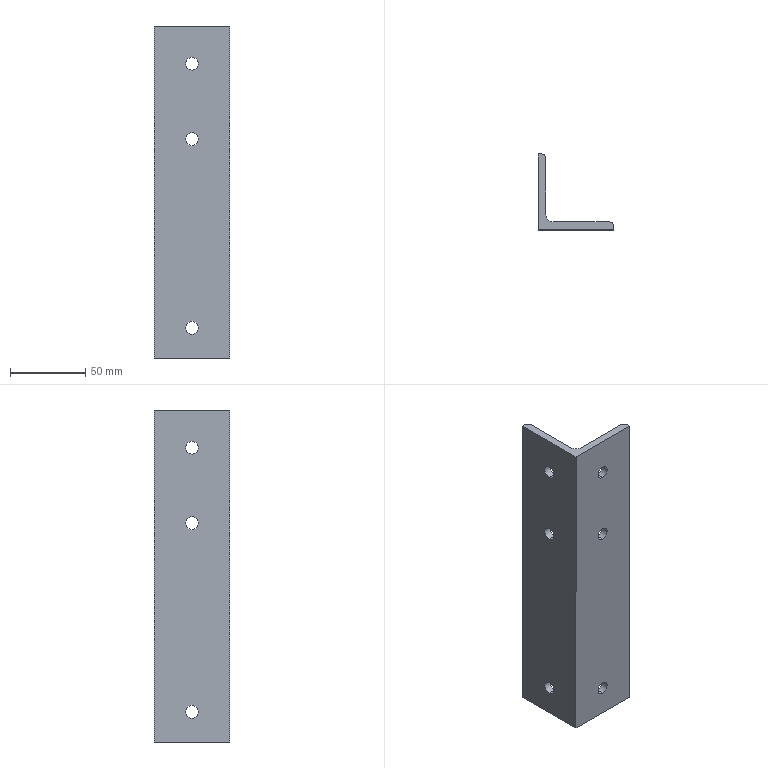Part | STEP file | 750038242 | 1 solid | 23 faces | box 50 x 50 x 220 mm | volume 103128 mm3 | cylinder 15 | plane 8 | commonest cylinder face diameters 8.5 x12 6 x2 10 x1
STEP:
#1=CARTESIAN_POINT('',(5.,25.,-94.25));
#2=VERTEX_POINT('',#1);
#3=CARTESIAN_POINT('',(5.,25.,-85.75));
#4=VERTEX_POINT('',#3);
#5=CARTESIAN_POINT('',(5.,25.,-90.));
#6=DIRECTION('',(-1.,0.,0.));
#7=DIRECTION('',(0.,0.,1.));
#8=AXIS2_PLACEMENT_3D('',#5,#6,#7);
#9=CIRCLE('',#8,4.25);
#10=EDGE_CURVE('',#2,#4,#9,.T.);
#11=ORIENTED_EDGE('',*,*,#10,.F.);
#12=CARTESIAN_POINT('',(0.,25.,-94.25));
#13=VERTEX_POINT('',#12);
#14=CARTESIAN_POINT('',(55.,25.,-94.25));
#15=DIRECTION('',(-1.,0.,0.));
#16=VECTOR('',#15,1000.);
#17=LINE('',#14,#16);
#18=EDGE_CURVE('',#2,#13,#17,.T.);
#19=ORIENTED_EDGE('',*,*,#18,.T.);
#20=CARTESIAN_POINT('',(0.,25.,-85.75));
#21=VERTEX_POINT('',#20);
#22=CARTESIAN_POINT('',(0.,25.,-90.));
#23=DIRECTION('',(-1.,0.,0.));
#24=DIRECTION('',(0.,0.,1.));
#25=AXIS2_PLACEMENT_3D('',#22,#23,#24);
#26=CIRCLE('',#25,4.25);
#27=EDGE_CURVE('',#13,#21,#26,.T.);
#28=ORIENTED_EDGE('',*,*,#27,.T.);
#29=CARTESIAN_POINT('',(55.,25.,-85.75));
#30=DIRECTION('',(-1.,0.,0.));
#31=VECTOR('',#30,1000.);
#32=LINE('',#29,#31);
#33=EDGE_CURVE('',#4,#21,#32,.T.);
#34=ORIENTED_EDGE('',*,*,#33,.F.);
#35=EDGE_LOOP('',(#11,#19,#28,#34));
#36=FACE_OUTER_BOUND('',#35,.T.);
#37=CARTESIAN_POINT('',(55.,25.,-90.));
#38=DIRECTION('',(-1.,0.,0.));
#39=DIRECTION('',(0.,0.,1.));
#40=AXIS2_PLACEMENT_3D('',#37,#38,#39);
#41=CYLINDRICAL_SURFACE('',#40,4.25);
#42=ADVANCED_FACE('',(#36),#41,.F.);
#43=CARTESIAN_POINT('',(5.,25.,30.75));
#44=VERTEX_POINT('',#43);
#45=CARTESIAN_POINT('',(5.,25.,39.25));
#46=VERTEX_POINT('',#45);
#47=CARTESIAN_POINT('',(5.,25.,35.));
#48=DIRECTION('',(-1.,0.,0.));
#49=DIRECTION('',(0.,0.,1.));
#50=AXIS2_PLACEMENT_3D('',#47,#48,#49);
#51=CIRCLE('',#50,4.25);
#52=EDGE_CURVE('',#44,#46,#51,.T.);
#53=ORIENTED_EDGE('',*,*,#52,.F.);
#54=CARTESIAN_POINT('',(0.,25.,30.75));
#55=VERTEX_POINT('',#54);
#56=CARTESIAN_POINT('',(55.,25.,30.75));
#57=DIRECTION('',(-1.,0.,0.));
#58=VECTOR('',#57,1000.);
#59=LINE('',#56,#58);
#60=EDGE_CURVE('',#44,#55,#59,.T.);
#61=ORIENTED_EDGE('',*,*,#60,.T.);
#62=CARTESIAN_POINT('',(0.,25.,39.25));
#63=VERTEX_POINT('',#62);
#64=CARTESIAN_POINT('',(0.,25.,35.));
#65=DIRECTION('',(-1.,0.,0.));
#66=DIRECTION('',(0.,0.,1.));
#67=AXIS2_PLACEMENT_3D('',#64,#65,#66);
#68=CIRCLE('',#67,4.25);
#69=EDGE_CURVE('',#55,#63,#68,.T.);
#70=ORIENTED_EDGE('',*,*,#69,.T.);
#71=CARTESIAN_POINT('',(55.,25.,39.25));
#72=DIRECTION('',(-1.,0.,0.));
#73=VECTOR('',#72,1000.);
#74=LINE('',#71,#73);
#75=EDGE_CURVE('',#46,#63,#74,.T.);
#76=ORIENTED_EDGE('',*,*,#75,.F.);
#77=EDGE_LOOP('',(#53,#61,#70,#76));
#78=FACE_OUTER_BOUND('',#77,.T.);
#79=CARTESIAN_POINT('',(55.,25.,35.));
#80=DIRECTION('',(-1.,0.,0.));
#81=DIRECTION('',(0.,0.,1.));
#82=AXIS2_PLACEMENT_3D('',#79,#80,#81);
#83=CYLINDRICAL_SURFACE('',#82,4.25);
#84=ADVANCED_FACE('',(#78),#83,.F.);
#85=CARTESIAN_POINT('',(5.,25.,80.75));
#86=VERTEX_POINT('',#85);
#87=CARTESIAN_POINT('',(5.,25.,89.25));
#88=VERTEX_POINT('',#87);
#89=CARTESIAN_POINT('',(5.,25.,85.));
#90=DIRECTION('',(-1.,0.,0.));
#91=DIRECTION('',(0.,0.,1.));
#92=AXIS2_PLACEMENT_3D('',#89,#90,#91);
#93=CIRCLE('',#92,4.25);
#94=EDGE_CURVE('',#86,#88,#93,.T.);
#95=ORIENTED_EDGE('',*,*,#94,.F.);
#96=CARTESIAN_POINT('',(0.,25.,80.75));
#97=VERTEX_POINT('',#96);
#98=CARTESIAN_POINT('',(55.,25.,80.75));
#99=DIRECTION('',(-1.,0.,0.));
#100=VECTOR('',#99,1000.);
#101=LINE('',#98,#100);
#102=EDGE_CURVE('',#86,#97,#101,.T.);
#103=ORIENTED_EDGE('',*,*,#102,.T.);
#104=CARTESIAN_POINT('',(0.,25.,89.25));
#105=VERTEX_POINT('',#104);
#106=CARTESIAN_POINT('',(0.,25.,85.));
#107=DIRECTION('',(-1.,0.,0.));
#108=DIRECTION('',(0.,0.,1.));
#109=AXIS2_PLACEMENT_3D('',#106,#107,#108);
#110=CIRCLE('',#109,4.25);
#111=EDGE_CURVE('',#97,#105,#110,.T.);
#112=ORIENTED_EDGE('',*,*,#111,.T.);
#113=CARTESIAN_POINT('',(55.,25.,89.25));
#114=DIRECTION('',(-1.,0.,0.));
#115=VECTOR('',#114,1000.);
#116=LINE('',#113,#115);
#117=EDGE_CURVE('',#88,#105,#116,.T.);
#118=ORIENTED_EDGE('',*,*,#117,.F.);
#119=EDGE_LOOP('',(#95,#103,#112,#118));
#120=FACE_OUTER_BOUND('',#119,.T.);
#121=CARTESIAN_POINT('',(55.,25.,85.));
#122=DIRECTION('',(-1.,0.,0.));
#123=DIRECTION('',(0.,0.,1.));
#124=AXIS2_PLACEMENT_3D('',#121,#122,#123);
#125=CYLINDRICAL_SURFACE('',#124,4.25);
#126=ADVANCED_FACE('',(#120),#125,.F.);
#127=CARTESIAN_POINT('',(25.,5.,-94.25));
#128=VERTEX_POINT('',#127);
#129=CARTESIAN_POINT('',(25.,5.,-85.75));
#130=VERTEX_POINT('',#129);
#131=CARTESIAN_POINT('',(25.,5.,-90.));
#132=DIRECTION('',(0.,1.,0.));
#133=DIRECTION('',(0.,0.,-1.));
#134=AXIS2_PLACEMENT_3D('',#131,#132,#133);
#135=CIRCLE('',#134,4.25);
#136=EDGE_CURVE('',#128,#130,#135,.T.);
#137=ORIENTED_EDGE('',*,*,#136,.T.);
#138=CARTESIAN_POINT('',(25.,0.,-85.75));
#139=VERTEX_POINT('',#138);
#140=CARTESIAN_POINT('',(25.,55.,-85.75));
#141=DIRECTION('',(0.,-1.,0.));
#142=VECTOR('',#141,1000.);
#143=LINE('',#140,#142);
#144=EDGE_CURVE('',#130,#139,#143,.T.);
#145=ORIENTED_EDGE('',*,*,#144,.T.);
#146=CARTESIAN_POINT('',(25.,0.,-94.25));
#147=VERTEX_POINT('',#146);
#148=CARTESIAN_POINT('',(25.,0.,-90.));
#149=DIRECTION('',(0.,-1.,0.));
#150=DIRECTION('',(0.,0.,-1.));
#151=AXIS2_PLACEMENT_3D('',#148,#149,#150);
#152=CIRCLE('',#151,4.25);
#153=EDGE_CURVE('',#139,#147,#152,.T.);
#154=ORIENTED_EDGE('',*,*,#153,.T.);
#155=CARTESIAN_POINT('',(25.,55.,-94.25));
#156=DIRECTION('',(0.,-1.,0.));
#157=VECTOR('',#156,1000.);
#158=LINE('',#155,#157);
#159=EDGE_CURVE('',#128,#147,#158,.T.);
#160=ORIENTED_EDGE('',*,*,#159,.F.);
#161=EDGE_LOOP('',(#137,#145,#154,#160));
#162=FACE_OUTER_BOUND('',#161,.T.);
#163=CARTESIAN_POINT('',(25.,55.,-90.));
#164=DIRECTION('',(0.,-1.,0.));
#165=DIRECTION('',(0.,0.,-1.));
#166=AXIS2_PLACEMENT_3D('',#163,#164,#165);
#167=CYLINDRICAL_SURFACE('',#166,4.25);
#168=ADVANCED_FACE('',(#162),#167,.F.);
#169=CARTESIAN_POINT('',(25.,5.,30.75));
#170=VERTEX_POINT('',#169);
#171=CARTESIAN_POINT('',(25.,5.,39.25));
#172=VERTEX_POINT('',#171);
#173=CARTESIAN_POINT('',(25.,5.,35.));
#174=DIRECTION('',(0.,1.,0.));
#175=DIRECTION('',(0.,0.,-1.));
#176=AXIS2_PLACEMENT_3D('',#173,#174,#175);
#177=CIRCLE('',#176,4.25);
#178=EDGE_CURVE('',#170,#172,#177,.T.);
#179=ORIENTED_EDGE('',*,*,#178,.T.);
#180=CARTESIAN_POINT('',(25.,0.,39.25));
#181=VERTEX_POINT('',#180);
#182=CARTESIAN_POINT('',(25.,55.,39.25));
#183=DIRECTION('',(0.,-1.,0.));
#184=VECTOR('',#183,1000.);
#185=LINE('',#182,#184);
#186=EDGE_CURVE('',#172,#181,#185,.T.);
#187=ORIENTED_EDGE('',*,*,#186,.T.);
#188=CARTESIAN_POINT('',(25.,0.,30.75));
#189=VERTEX_POINT('',#188);
#190=CARTESIAN_POINT('',(25.,0.,35.));
#191=DIRECTION('',(0.,-1.,0.));
#192=DIRECTION('',(0.,0.,-1.));
#193=AXIS2_PLACEMENT_3D('',#190,#191,#192);
#194=CIRCLE('',#193,4.25);
#195=EDGE_CURVE('',#181,#189,#194,.T.);
#196=ORIENTED_EDGE('',*,*,#195,.T.);
#197=CARTESIAN_POINT('',(25.,55.,30.75));
#198=DIRECTION('',(0.,-1.,0.));
#199=VECTOR('',#198,1000.);
#200=LINE('',#197,#199);
#201=EDGE_CURVE('',#170,#189,#200,.T.);
#202=ORIENTED_EDGE('',*,*,#201,.F.);
#203=EDGE_LOOP('',(#179,#187,#196,#202));
#204=FACE_OUTER_BOUND('',#203,.T.);
#205=CARTESIAN_POINT('',(25.,55.,35.));
#206=DIRECTION('',(0.,-1.,0.));
#207=DIRECTION('',(0.,0.,-1.));
#208=AXIS2_PLACEMENT_3D('',#205,#206,#207);
#209=CYLINDRICAL_SURFACE('',#208,4.25);
#210=ADVANCED_FACE('',(#204),#209,.F.);
#211=CARTESIAN_POINT('',(25.,5.,80.75));
#212=VERTEX_POINT('',#211);
#213=CARTESIAN_POINT('',(25.,5.,89.25));
#214=VERTEX_POINT('',#213);
#215=CARTESIAN_POINT('',(25.,5.,85.));
#216=DIRECTION('',(0.,1.,0.));
#217=DIRECTION('',(0.,0.,-1.));
#218=AXIS2_PLACEMENT_3D('',#215,#216,#217);
#219=CIRCLE('',#218,4.25);
#220=EDGE_CURVE('',#212,#214,#219,.T.);
#221=ORIENTED_EDGE('',*,*,#220,.T.);
#222=CARTESIAN_POINT('',(25.,0.,89.25));
#223=VERTEX_POINT('',#222);
#224=CARTESIAN_POINT('',(25.,55.,89.25));
#225=DIRECTION('',(0.,-1.,0.));
#226=VECTOR('',#225,1000.);
#227=LINE('',#224,#226);
#228=EDGE_CURVE('',#214,#223,#227,.T.);
#229=ORIENTED_EDGE('',*,*,#228,.T.);
#230=CARTESIAN_POINT('',(25.,0.,80.75));
#231=VERTEX_POINT('',#230);
#232=CARTESIAN_POINT('',(25.,0.,85.));
#233=DIRECTION('',(0.,-1.,0.));
#234=DIRECTION('',(0.,0.,-1.));
#235=AXIS2_PLACEMENT_3D('',#232,#233,#234);
#236=CIRCLE('',#235,4.25);
#237=EDGE_CURVE('',#223,#231,#236,.T.);
#238=ORIENTED_EDGE('',*,*,#237,.T.);
#239=CARTESIAN_POINT('',(25.,55.,80.75));
#240=DIRECTION('',(0.,-1.,0.));
#241=VECTOR('',#240,1000.);
#242=LINE('',#239,#241);
#243=EDGE_CURVE('',#212,#231,#242,.T.);
#244=ORIENTED_EDGE('',*,*,#243,.F.);
#245=EDGE_LOOP('',(#221,#229,#238,#244));
#246=FACE_OUTER_BOUND('',#245,.T.);
#247=CARTESIAN_POINT('',(25.,55.,85.));
#248=DIRECTION('',(0.,-1.,0.));
#249=DIRECTION('',(0.,0.,-1.));
#250=AXIS2_PLACEMENT_3D('',#247,#248,#249);
#251=CYLINDRICAL_SURFACE('',#250,4.25);
#252=ADVANCED_FACE('',(#246),#251,.F.);
#253=CARTESIAN_POINT('',(0.,25.,-90.));
#254=DIRECTION('',(-1.,0.,0.));
#255=DIRECTION('',(0.,0.,1.));
#256=AXIS2_PLACEMENT_3D('',#253,#254,#255);
#257=CIRCLE('',#256,4.25);
#258=EDGE_CURVE('',#21,#13,#257,.T.);
#259=ORIENTED_EDGE('',*,*,#258,.F.);
#260=ORIENTED_EDGE('',*,*,#27,.F.);
#261=EDGE_LOOP('',(#259,#260));
#262=FACE_BOUND('',#261,.T.);
#263=CARTESIAN_POINT('',(0.,25.,35.));
#264=DIRECTION('',(-1.,0.,0.));
#265=DIRECTION('',(0.,0.,1.));
#266=AXIS2_PLACEMENT_3D('',#263,#264,#265);
#267=CIRCLE('',#266,4.25);
#268=EDGE_CURVE('',#63,#55,#267,.T.);
#269=ORIENTED_EDGE('',*,*,#268,.F.);
#270=ORIENTED_EDGE('',*,*,#69,.F.);
#271=EDGE_LOOP('',(#269,#270));
#272=FACE_BOUND('',#271,.T.);
#273=CARTESIAN_POINT('',(0.,0.,110.));
#274=VERTEX_POINT('',#273);
#275=CARTESIAN_POINT('',(0.,0.,-110.));
#276=VERTEX_POINT('',#275);
#277=CARTESIAN_POINT('',(0.,0.,110.));
#278=DIRECTION('',(0.,0.,-1.));
#279=VECTOR('',#278,1000.);
#280=LINE('',#277,#279);
#281=EDGE_CURVE('',#274,#276,#280,.T.);
#282=ORIENTED_EDGE('',*,*,#281,.F.);
#283=CARTESIAN_POINT('',(0.,50.,110.));
#284=VERTEX_POINT('',#283);
#285=CARTESIAN_POINT('',(0.,50.,110.));
#286=DIRECTION('',(0.,-1.,0.));
#287=VECTOR('',#286,1000.);
#288=LINE('',#285,#287);
#289=EDGE_CURVE('',#284,#274,#288,.T.);
#290=ORIENTED_EDGE('',*,*,#289,.F.);
#291=CARTESIAN_POINT('',(0.,50.,-110.));
#292=VERTEX_POINT('',#291);
#293=CARTESIAN_POINT('',(0.,50.,110.));
#294=DIRECTION('',(0.,0.,1.));
#295=VECTOR('',#294,1000.);
#296=LINE('',#293,#295);
#297=EDGE_CURVE('',#292,#284,#296,.T.);
#298=ORIENTED_EDGE('',*,*,#297,.F.);
#299=CARTESIAN_POINT('',(0.,50.,-110.));
#300=DIRECTION('',(0.,1.,0.));
#301=VECTOR('',#300,1000.);
#302=LINE('',#299,#301);
#303=EDGE_CURVE('',#276,#292,#302,.T.);
#304=ORIENTED_EDGE('',*,*,#303,.F.);
#305=EDGE_LOOP('',(#282,#290,#298,#304));
#306=FACE_OUTER_BOUND('',#305,.T.);
#307=CARTESIAN_POINT('',(0.,25.,85.));
#308=DIRECTION('',(-1.,0.,0.));
#309=DIRECTION('',(0.,0.,1.));
#310=AXIS2_PLACEMENT_3D('',#307,#308,#309);
#311=CIRCLE('',#310,4.25);
#312=EDGE_CURVE('',#105,#97,#311,.T.);
#313=ORIENTED_EDGE('',*,*,#312,.F.);
#314=ORIENTED_EDGE('',*,*,#111,.F.);
#315=EDGE_LOOP('',(#313,#314));
#316=FACE_BOUND('',#315,.T.);
#317=CARTESIAN_POINT('',(0.,50.,110.));
#318=DIRECTION('',(1.,0.,0.));
#319=DIRECTION('',(0.,1.,0.));
#320=AXIS2_PLACEMENT_3D('',#317,#318,#319);
#321=PLANE('',#320);
#322=ADVANCED_FACE('',(#262,#272,#306,#316),#321,.F.);
#323=ORIENTED_EDGE('',*,*,#18,.F.);
#324=CARTESIAN_POINT('',(5.,25.,-90.));
#325=DIRECTION('',(-1.,0.,0.));
#326=DIRECTION('',(0.,0.,1.));
#327=AXIS2_PLACEMENT_3D('',#324,#325,#326);
#328=CIRCLE('',#327,4.25);
#329=EDGE_CURVE('',#4,#2,#328,.T.);
#330=ORIENTED_EDGE('',*,*,#329,.F.);
#331=ORIENTED_EDGE('',*,*,#33,.T.);
#332=ORIENTED_EDGE('',*,*,#258,.T.);
#333=EDGE_LOOP('',(#323,#330,#331,#332));
#334=FACE_OUTER_BOUND('',#333,.T.);
#335=CARTESIAN_POINT('',(55.,25.,-90.));
#336=DIRECTION('',(-1.,0.,0.));
#337=DIRECTION('',(0.,0.,1.));
#338=AXIS2_PLACEMENT_3D('',#335,#336,#337);
#339=CYLINDRICAL_SURFACE('',#338,4.25);
#340=ADVANCED_FACE('',(#334),#339,.F.);
#341=ORIENTED_EDGE('',*,*,#60,.F.);
#342=CARTESIAN_POINT('',(5.,25.,35.));
#343=DIRECTION('',(-1.,0.,0.));
#344=DIRECTION('',(0.,0.,1.));
#345=AXIS2_PLACEMENT_3D('',#342,#343,#344);
#346=CIRCLE('',#345,4.25);
#347=EDGE_CURVE('',#46,#44,#346,.T.);
#348=ORIENTED_EDGE('',*,*,#347,.F.);
#349=ORIENTED_EDGE('',*,*,#75,.T.);
#350=ORIENTED_EDGE('',*,*,#268,.T.);
#351=EDGE_LOOP('',(#341,#348,#349,#350));
#352=FACE_OUTER_BOUND('',#351,.T.);
#353=CARTESIAN_POINT('',(55.,25.,35.));
#354=DIRECTION('',(-1.,0.,0.));
#355=DIRECTION('',(0.,0.,1.));
#356=AXIS2_PLACEMENT_3D('',#353,#354,#355);
#357=CYLINDRICAL_SURFACE('',#356,4.25);
#358=ADVANCED_FACE('',(#352),#357,.F.);
#359=CARTESIAN_POINT('',(2.,50.,-110.));
#360=VERTEX_POINT('',#359);
#361=CARTESIAN_POINT('',(47.,50.,-110.));
#362=DIRECTION('',(-1.,0.,0.));
#363=VECTOR('',#362,1000.);
#364=LINE('',#361,#363);
#365=EDGE_CURVE('',#360,#292,#364,.T.);
#366=ORIENTED_EDGE('',*,*,#365,.F.);
#367=CARTESIAN_POINT('',(5.,47.,-110.));
#368=VERTEX_POINT('',#367);
#369=CARTESIAN_POINT('',(2.,47.,-110.));
#370=DIRECTION('',(0.,0.,1.));
#371=DIRECTION('',(-1.,0.,0.));
#372=AXIS2_PLACEMENT_3D('',#369,#370,#371);
#373=CIRCLE('',#372,3.);
#374=EDGE_CURVE('',#368,#360,#373,.T.);
#375=ORIENTED_EDGE('',*,*,#374,.F.);
#376=CARTESIAN_POINT('',(5.,10.,-110.));
#377=VERTEX_POINT('',#376);
#378=CARTESIAN_POINT('',(5.,2.,-110.));
#379=DIRECTION('',(0.,1.,0.));
#380=VECTOR('',#379,1000.);
#381=LINE('',#378,#380);
#382=EDGE_CURVE('',#377,#368,#381,.T.);
#383=ORIENTED_EDGE('',*,*,#382,.F.);
#384=CARTESIAN_POINT('',(10.,5.,-110.));
#385=VERTEX_POINT('',#384);
#386=CARTESIAN_POINT('',(10.,10.,-110.));
#387=DIRECTION('',(0.,0.,-1.));
#388=DIRECTION('',(-1.,0.,0.));
#389=AXIS2_PLACEMENT_3D('',#386,#387,#388);
#390=CIRCLE('',#389,5.);
#391=EDGE_CURVE('',#385,#377,#390,.T.);
#392=ORIENTED_EDGE('',*,*,#391,.F.);
#393=CARTESIAN_POINT('',(47.,5.,-110.));
#394=VERTEX_POINT('',#393);
#395=CARTESIAN_POINT('',(47.,5.,-110.));
#396=DIRECTION('',(-1.,0.,0.));
#397=VECTOR('',#396,1000.);
#398=LINE('',#395,#397);
#399=EDGE_CURVE('',#394,#385,#398,.T.);
#400=ORIENTED_EDGE('',*,*,#399,.F.);
#401=CARTESIAN_POINT('',(50.,2.,-110.));
#402=VERTEX_POINT('',#401);
#403=CARTESIAN_POINT('',(47.,2.,-110.));
#404=DIRECTION('',(0.,0.,1.));
#405=DIRECTION('',(-1.,0.,0.));
#406=AXIS2_PLACEMENT_3D('',#403,#404,#405);
#407=CIRCLE('',#406,3.);
#408=EDGE_CURVE('',#402,#394,#407,.T.);
#409=ORIENTED_EDGE('',*,*,#408,.F.);
#410=CARTESIAN_POINT('',(50.,0.,-110.));
#411=VERTEX_POINT('',#410);
#412=CARTESIAN_POINT('',(50.,2.,-110.));
#413=DIRECTION('',(0.,1.,0.));
#414=VECTOR('',#413,1000.);
#415=LINE('',#412,#414);
#416=EDGE_CURVE('',#411,#402,#415,.T.);
#417=ORIENTED_EDGE('',*,*,#416,.F.);
#418=CARTESIAN_POINT('',(47.,0.,-110.));
#419=DIRECTION('',(1.,0.,0.));
#420=VECTOR('',#419,1000.);
#421=LINE('',#418,#420);
#422=EDGE_CURVE('',#276,#411,#421,.T.);
#423=ORIENTED_EDGE('',*,*,#422,.F.);
#424=ORIENTED_EDGE('',*,*,#303,.T.);
#425=EDGE_LOOP('',(#366,#375,#383,#392,#400,#409,#417,#423,#424));
#426=FACE_OUTER_BOUND('',#425,.T.);
#427=CARTESIAN_POINT('',(47.,2.,-110.));
#428=DIRECTION('',(0.,0.,1.));
#429=DIRECTION('',(1.,0.,0.));
#430=AXIS2_PLACEMENT_3D('',#427,#428,#429);
#431=PLANE('',#430);
#432=ADVANCED_FACE('',(#426),#431,.F.);
#433=CARTESIAN_POINT('',(25.,0.,-90.));
#434=DIRECTION('',(0.,-1.,0.));
#435=DIRECTION('',(0.,0.,-1.));
#436=AXIS2_PLACEMENT_3D('',#433,#434,#435);
#437=CIRCLE('',#436,4.25);
#438=EDGE_CURVE('',#147,#139,#437,.T.);
#439=ORIENTED_EDGE('',*,*,#438,.F.);
#440=ORIENTED_EDGE('',*,*,#153,.F.);
#441=EDGE_LOOP('',(#439,#440));
#442=FACE_BOUND('',#441,.T.);
#443=CARTESIAN_POINT('',(25.,0.,35.));
#444=DIRECTION('',(0.,-1.,0.));
#445=DIRECTION('',(0.,0.,-1.));
#446=AXIS2_PLACEMENT_3D('',#443,#444,#445);
#447=CIRCLE('',#446,4.25);
#448=EDGE_CURVE('',#189,#181,#447,.T.);
#449=ORIENTED_EDGE('',*,*,#448,.F.);
#450=ORIENTED_EDGE('',*,*,#195,.F.);
#451=EDGE_LOOP('',(#449,#450));
#452=FACE_BOUND('',#451,.T.);
#453=CARTESIAN_POINT('',(50.,0.,110.));
#454=VERTEX_POINT('',#453);
#455=CARTESIAN_POINT('',(50.,0.,110.));
#456=DIRECTION('',(0.,0.,-1.));
#457=VECTOR('',#456,1000.);
#458=LINE('',#455,#457);
#459=EDGE_CURVE('',#454,#411,#458,.T.);
#460=ORIENTED_EDGE('',*,*,#459,.F.);
#461=CARTESIAN_POINT('',(0.,0.,110.));
#462=DIRECTION('',(1.,0.,0.));
#463=VECTOR('',#462,1000.);
#464=LINE('',#461,#463);
#465=EDGE_CURVE('',#274,#454,#464,.T.);
#466=ORIENTED_EDGE('',*,*,#465,.F.);
#467=ORIENTED_EDGE('',*,*,#281,.T.);
#468=ORIENTED_EDGE('',*,*,#422,.T.);
#469=EDGE_LOOP('',(#460,#466,#467,#468));
#470=FACE_OUTER_BOUND('',#469,.T.);
#471=CARTESIAN_POINT('',(25.,0.,85.));
#472=DIRECTION('',(0.,-1.,0.));
#473=DIRECTION('',(0.,0.,-1.));
#474=AXIS2_PLACEMENT_3D('',#471,#472,#473);
#475=CIRCLE('',#474,4.25);
#476=EDGE_CURVE('',#231,#223,#475,.T.);
#477=ORIENTED_EDGE('',*,*,#476,.F.);
#478=ORIENTED_EDGE('',*,*,#237,.F.);
#479=EDGE_LOOP('',(#477,#478));
#480=FACE_BOUND('',#479,.T.);
#481=CARTESIAN_POINT('',(0.,0.,110.));
#482=DIRECTION('',(0.,1.,0.));
#483=DIRECTION('',(0.,0.,1.));
#484=AXIS2_PLACEMENT_3D('',#481,#482,#483);
#485=PLANE('',#484);
#486=ADVANCED_FACE('',(#442,#452,#470,#480),#485,.F.);
#487=CARTESIAN_POINT('',(5.,47.,110.));
#488=VERTEX_POINT('',#487);
#489=CARTESIAN_POINT('',(2.,50.,110.));
#490=VERTEX_POINT('',#489);
#491=CARTESIAN_POINT('',(2.,47.,110.));
#492=DIRECTION('',(0.,0.,1.));
#493=DIRECTION('',(-1.,0.,0.));
#494=AXIS2_PLACEMENT_3D('',#491,#492,#493);
#495=CIRCLE('',#494,3.);
#496=EDGE_CURVE('',#488,#490,#495,.T.);
#497=ORIENTED_EDGE('',*,*,#496,.T.);
#498=CARTESIAN_POINT('',(47.,50.,110.));
#499=DIRECTION('',(-1.,0.,0.));
#500=VECTOR('',#499,1000.);
#501=LINE('',#498,#500);
#502=EDGE_CURVE('',#490,#284,#501,.T.);
#503=ORIENTED_EDGE('',*,*,#502,.T.);
#504=ORIENTED_EDGE('',*,*,#289,.T.);
#505=ORIENTED_EDGE('',*,*,#465,.T.);
#506=CARTESIAN_POINT('',(50.,2.,110.));
#507=VERTEX_POINT('',#506);
#508=CARTESIAN_POINT('',(50.,2.,110.));
#509=DIRECTION('',(0.,1.,0.));
#510=VECTOR('',#509,1000.);
#511=LINE('',#508,#510);
#512=EDGE_CURVE('',#454,#507,#511,.T.);
#513=ORIENTED_EDGE('',*,*,#512,.T.);
#514=CARTESIAN_POINT('',(47.,5.,110.));
#515=VERTEX_POINT('',#514);
#516=CARTESIAN_POINT('',(47.,2.,110.));
#517=DIRECTION('',(0.,0.,1.));
#518=DIRECTION('',(-1.,0.,0.));
#519=AXIS2_PLACEMENT_3D('',#516,#517,#518);
#520=CIRCLE('',#519,3.);
#521=EDGE_CURVE('',#507,#515,#520,.T.);
#522=ORIENTED_EDGE('',*,*,#521,.T.);
#523=CARTESIAN_POINT('',(10.,5.,110.));
#524=VERTEX_POINT('',#523);
#525=CARTESIAN_POINT('',(47.,5.,110.));
#526=DIRECTION('',(-1.,0.,0.));
#527=VECTOR('',#526,1000.);
#528=LINE('',#525,#527);
#529=EDGE_CURVE('',#515,#524,#528,.T.);
#530=ORIENTED_EDGE('',*,*,#529,.T.);
#531=CARTESIAN_POINT('',(5.,10.,110.));
#532=VERTEX_POINT('',#531);
#533=CARTESIAN_POINT('',(10.,10.,110.));
#534=DIRECTION('',(0.,0.,-1.));
#535=DIRECTION('',(-1.,0.,0.));
#536=AXIS2_PLACEMENT_3D('',#533,#534,#535);
#537=CIRCLE('',#536,5.);
#538=EDGE_CURVE('',#524,#532,#537,.T.);
#539=ORIENTED_EDGE('',*,*,#538,.T.);
#540=CARTESIAN_POINT('',(5.,2.,110.));
#541=DIRECTION('',(0.,1.,0.));
#542=VECTOR('',#541,1000.);
#543=LINE('',#540,#542);
#544=EDGE_CURVE('',#532,#488,#543,.T.);
#545=ORIENTED_EDGE('',*,*,#544,.T.);
#546=EDGE_LOOP('',(#497,#503,#504,#505,#513,#522,#530,#539,#545));
#547=FACE_OUTER_BOUND('',#546,.T.);
#548=CARTESIAN_POINT('',(47.,2.,110.));
#549=DIRECTION('',(0.,0.,1.));
#550=DIRECTION('',(1.,0.,0.));
#551=AXIS2_PLACEMENT_3D('',#548,#549,#550);
#552=PLANE('',#551);
#553=ADVANCED_FACE('',(#547),#552,.T.);
#554=ORIENTED_EDGE('',*,*,#297,.T.);
#555=ORIENTED_EDGE('',*,*,#502,.F.);
#556=CARTESIAN_POINT('',(2.,50.,110.));
#557=DIRECTION('',(0.,0.,1.));
#558=VECTOR('',#557,1000.);
#559=LINE('',#556,#558);
#560=EDGE_CURVE('',#360,#490,#559,.T.);
#561=ORIENTED_EDGE('',*,*,#560,.F.);
#562=ORIENTED_EDGE('',*,*,#365,.T.);
#563=EDGE_LOOP('',(#554,#555,#561,#562));
#564=FACE_OUTER_BOUND('',#563,.T.);
#565=CARTESIAN_POINT('',(2.,50.,110.));
#566=DIRECTION('',(0.,-1.,0.));
#567=DIRECTION('',(0.,0.,-1.));
#568=AXIS2_PLACEMENT_3D('',#565,#566,#567);
#569=PLANE('',#568);
#570=ADVANCED_FACE('',(#564),#569,.F.);
#571=ORIENTED_EDGE('',*,*,#102,.F.);
#572=CARTESIAN_POINT('',(5.,25.,85.));
#573=DIRECTION('',(-1.,0.,0.));
#574=DIRECTION('',(0.,0.,1.));
#575=AXIS2_PLACEMENT_3D('',#572,#573,#574);
#576=CIRCLE('',#575,4.25);
#577=EDGE_CURVE('',#88,#86,#576,.T.);
#578=ORIENTED_EDGE('',*,*,#577,.F.);
#579=ORIENTED_EDGE('',*,*,#117,.T.);
#580=ORIENTED_EDGE('',*,*,#312,.T.);
#581=EDGE_LOOP('',(#571,#578,#579,#580));
#582=FACE_OUTER_BOUND('',#581,.T.);
#583=CARTESIAN_POINT('',(55.,25.,85.));
#584=DIRECTION('',(-1.,0.,0.));
#585=DIRECTION('',(0.,0.,1.));
#586=AXIS2_PLACEMENT_3D('',#583,#584,#585);
#587=CYLINDRICAL_SURFACE('',#586,4.25);
#588=ADVANCED_FACE('',(#582),#587,.F.);
#589=ORIENTED_EDGE('',*,*,#329,.T.);
#590=ORIENTED_EDGE('',*,*,#10,.T.);
#591=EDGE_LOOP('',(#589,#590));
#592=FACE_BOUND('',#591,.T.);
#593=CARTESIAN_POINT('',(5.,47.,110.));
#594=DIRECTION('',(0.,0.,-1.));
#595=VECTOR('',#594,1000.);
#596=LINE('',#593,#595);
#597=EDGE_CURVE('',#488,#368,#596,.T.);
#598=ORIENTED_EDGE('',*,*,#597,.F.);
#599=ORIENTED_EDGE('',*,*,#544,.F.);
#600=CARTESIAN_POINT('',(5.,10.,110.));
#601=DIRECTION('',(0.,0.,1.));
#602=VECTOR('',#601,1000.);
#603=LINE('',#600,#602);
#604=EDGE_CURVE('',#377,#532,#603,.T.);
#605=ORIENTED_EDGE('',*,*,#604,.F.);
#606=ORIENTED_EDGE('',*,*,#382,.T.);
#607=EDGE_LOOP('',(#598,#599,#605,#606));
#608=FACE_OUTER_BOUND('',#607,.T.);
#609=ORIENTED_EDGE('',*,*,#347,.T.);
#610=ORIENTED_EDGE('',*,*,#52,.T.);
#611=EDGE_LOOP('',(#609,#610));
#612=FACE_BOUND('',#611,.T.);
#613=ORIENTED_EDGE('',*,*,#577,.T.);
#614=ORIENTED_EDGE('',*,*,#94,.T.);
#615=EDGE_LOOP('',(#613,#614));
#616=FACE_BOUND('',#615,.T.);
#617=CARTESIAN_POINT('',(5.,10.,110.));
#618=DIRECTION('',(-1.,0.,0.));
#619=DIRECTION('',(0.,-1.,0.));
#620=AXIS2_PLACEMENT_3D('',#617,#618,#619);
#621=PLANE('',#620);
#622=ADVANCED_FACE('',(#592,#608,#612,#616),#621,.F.);
#623=ORIENTED_EDGE('',*,*,#496,.F.);
#624=ORIENTED_EDGE('',*,*,#597,.T.);
#625=ORIENTED_EDGE('',*,*,#374,.T.);
#626=ORIENTED_EDGE('',*,*,#560,.T.);
#627=EDGE_LOOP('',(#623,#624,#625,#626));
#628=FACE_OUTER_BOUND('',#627,.T.);
#629=CARTESIAN_POINT('',(2.,47.,110.));
#630=DIRECTION('',(0.,0.,-1.));
#631=DIRECTION('',(-1.,0.,0.));
#632=AXIS2_PLACEMENT_3D('',#629,#630,#631);
#633=CYLINDRICAL_SURFACE('',#632,3.);
#634=ADVANCED_FACE('',(#628),#633,.T.);
#635=ORIENTED_EDGE('',*,*,#604,.T.);
#636=ORIENTED_EDGE('',*,*,#538,.F.);
#637=CARTESIAN_POINT('',(10.,5.,110.));
#638=DIRECTION('',(0.,0.,1.));
#639=VECTOR('',#638,1000.);
#640=LINE('',#637,#639);
#641=EDGE_CURVE('',#385,#524,#640,.T.);
#642=ORIENTED_EDGE('',*,*,#641,.F.);
#643=ORIENTED_EDGE('',*,*,#391,.T.);
#644=EDGE_LOOP('',(#635,#636,#642,#643));
#645=FACE_OUTER_BOUND('',#644,.T.);
#646=CARTESIAN_POINT('',(10.,10.,110.));
#647=DIRECTION('',(0.,0.,-1.));
#648=DIRECTION('',(-1.,0.,0.));
#649=AXIS2_PLACEMENT_3D('',#646,#647,#648);
#650=CYLINDRICAL_SURFACE('',#649,5.);
#651=ADVANCED_FACE('',(#645),#650,.F.);
#652=ORIENTED_EDGE('',*,*,#136,.F.);
#653=CARTESIAN_POINT('',(25.,5.,-90.));
#654=DIRECTION('',(0.,1.,0.));
#655=DIRECTION('',(0.,0.,-1.));
#656=AXIS2_PLACEMENT_3D('',#653,#654,#655);
#657=CIRCLE('',#656,4.25);
#658=EDGE_CURVE('',#130,#128,#657,.T.);
#659=ORIENTED_EDGE('',*,*,#658,.F.);
#660=EDGE_LOOP('',(#652,#659));
#661=FACE_BOUND('',#660,.T.);
#662=ORIENTED_EDGE('',*,*,#641,.T.);
#663=ORIENTED_EDGE('',*,*,#529,.F.);
#664=CARTESIAN_POINT('',(47.,5.,110.));
#665=DIRECTION('',(0.,0.,1.));
#666=VECTOR('',#665,1000.);
#667=LINE('',#664,#666);
#668=EDGE_CURVE('',#394,#515,#667,.T.);
#669=ORIENTED_EDGE('',*,*,#668,.F.);
#670=ORIENTED_EDGE('',*,*,#399,.T.);
#671=EDGE_LOOP('',(#662,#663,#669,#670));
#672=FACE_OUTER_BOUND('',#671,.T.);
#673=ORIENTED_EDGE('',*,*,#178,.F.);
#674=CARTESIAN_POINT('',(25.,5.,35.));
#675=DIRECTION('',(0.,1.,0.));
#676=DIRECTION('',(0.,0.,-1.));
#677=AXIS2_PLACEMENT_3D('',#674,#675,#676);
#678=CIRCLE('',#677,4.25);
#679=EDGE_CURVE('',#172,#170,#678,.T.);
#680=ORIENTED_EDGE('',*,*,#679,.F.);
#681=EDGE_LOOP('',(#673,#680));
#682=FACE_BOUND('',#681,.T.);
#683=ORIENTED_EDGE('',*,*,#220,.F.);
#684=CARTESIAN_POINT('',(25.,5.,85.));
#685=DIRECTION('',(0.,1.,0.));
#686=DIRECTION('',(0.,0.,-1.));
#687=AXIS2_PLACEMENT_3D('',#684,#685,#686);
#688=CIRCLE('',#687,4.25);
#689=EDGE_CURVE('',#214,#212,#688,.T.);
#690=ORIENTED_EDGE('',*,*,#689,.F.);
#691=EDGE_LOOP('',(#683,#690));
#692=FACE_BOUND('',#691,.T.);
#693=CARTESIAN_POINT('',(47.,5.,110.));
#694=DIRECTION('',(0.,-1.,0.));
#695=DIRECTION('',(0.,0.,-1.));
#696=AXIS2_PLACEMENT_3D('',#693,#694,#695);
#697=PLANE('',#696);
#698=ADVANCED_FACE('',(#661,#672,#682,#692),#697,.F.);
#699=ORIENTED_EDGE('',*,*,#521,.F.);
#700=CARTESIAN_POINT('',(50.,2.,110.));
#701=DIRECTION('',(0.,0.,-1.));
#702=VECTOR('',#701,1000.);
#703=LINE('',#700,#702);
#704=EDGE_CURVE('',#507,#402,#703,.T.);
#705=ORIENTED_EDGE('',*,*,#704,.T.);
#706=ORIENTED_EDGE('',*,*,#408,.T.);
#707=ORIENTED_EDGE('',*,*,#668,.T.);
#708=EDGE_LOOP('',(#699,#705,#706,#707));
#709=FACE_OUTER_BOUND('',#708,.T.);
#710=CARTESIAN_POINT('',(47.,2.,110.));
#711=DIRECTION('',(0.,0.,-1.));
#712=DIRECTION('',(-1.,0.,0.));
#713=AXIS2_PLACEMENT_3D('',#710,#711,#712);
#714=CYLINDRICAL_SURFACE('',#713,3.);
#715=ADVANCED_FACE('',(#709),#714,.T.);
#716=ORIENTED_EDGE('',*,*,#704,.F.);
#717=ORIENTED_EDGE('',*,*,#512,.F.);
#718=ORIENTED_EDGE('',*,*,#459,.T.);
#719=ORIENTED_EDGE('',*,*,#416,.T.);
#720=EDGE_LOOP('',(#716,#717,#718,#719));
#721=FACE_OUTER_BOUND('',#720,.T.);
#722=CARTESIAN_POINT('',(50.,0.,110.));
#723=DIRECTION('',(-1.,0.,0.));
#724=DIRECTION('',(0.,0.,1.));
#725=AXIS2_PLACEMENT_3D('',#722,#723,#724);
#726=PLANE('',#725);
#727=ADVANCED_FACE('',(#721),#726,.F.);
#728=ORIENTED_EDGE('',*,*,#144,.F.);
#729=ORIENTED_EDGE('',*,*,#658,.T.);
#730=ORIENTED_EDGE('',*,*,#159,.T.);
#731=ORIENTED_EDGE('',*,*,#438,.T.);
#732=EDGE_LOOP('',(#728,#729,#730,#731));
#733=FACE_OUTER_BOUND('',#732,.T.);
#734=CARTESIAN_POINT('',(25.,55.,-90.));
#735=DIRECTION('',(0.,-1.,0.));
#736=DIRECTION('',(0.,0.,-1.));
#737=AXIS2_PLACEMENT_3D('',#734,#735,#736);
#738=CYLINDRICAL_SURFACE('',#737,4.25);
#739=ADVANCED_FACE('',(#733),#738,.F.);
#740=ORIENTED_EDGE('',*,*,#186,.F.);
#741=ORIENTED_EDGE('',*,*,#679,.T.);
#742=ORIENTED_EDGE('',*,*,#201,.T.);
#743=ORIENTED_EDGE('',*,*,#448,.T.);
#744=EDGE_LOOP('',(#740,#741,#742,#743));
#745=FACE_OUTER_BOUND('',#744,.T.);
#746=CARTESIAN_POINT('',(25.,55.,35.));
#747=DIRECTION('',(0.,-1.,0.));
#748=DIRECTION('',(0.,0.,-1.));
#749=AXIS2_PLACEMENT_3D('',#746,#747,#748);
#750=CYLINDRICAL_SURFACE('',#749,4.25);
#751=ADVANCED_FACE('',(#745),#750,.F.);
#752=ORIENTED_EDGE('',*,*,#228,.F.);
#753=ORIENTED_EDGE('',*,*,#689,.T.);
#754=ORIENTED_EDGE('',*,*,#243,.T.);
#755=ORIENTED_EDGE('',*,*,#476,.T.);
#756=EDGE_LOOP('',(#752,#753,#754,#755));
#757=FACE_OUTER_BOUND('',#756,.T.);
#758=CARTESIAN_POINT('',(25.,55.,85.));
#759=DIRECTION('',(0.,-1.,0.));
#760=DIRECTION('',(0.,0.,-1.));
#761=AXIS2_PLACEMENT_3D('',#758,#759,#760);
#762=CYLINDRICAL_SURFACE('',#761,4.25);
#763=ADVANCED_FACE('',(#757),#762,.F.);
#764=CLOSED_SHELL('',(#42,#84,#126,#168,#210,#252,#322,#340,#358,#432,#486,#553,#570,#588,#622,#634,#651,#698,#715,#727,#739,#751,#763));
#765=MANIFOLD_SOLID_BREP('',#764);
#766=CARTESIAN_POINT('',(0.,0.,0.));
#767=DIRECTION('',(0.,0.,1.));
#768=DIRECTION('',(1.,0.,0.));
#769=AXIS2_PLACEMENT_3D('',#766,#767,#768);
#770=(LENGTH_UNIT()NAMED_UNIT(*)SI_UNIT(.MILLI.,.METRE.));
#771=UNCERTAINTY_MEASURE_WITH_UNIT(LENGTH_MEASURE(0.00001),#770,'','');
#772=(NAMED_UNIT(*)PLANE_ANGLE_UNIT()SI_UNIT($,.RADIAN.));
#773=(NAMED_UNIT(*)SI_UNIT($,.STERADIAN.)SOLID_ANGLE_UNIT());
#774=(GEOMETRIC_REPRESENTATION_CONTEXT(3)GLOBAL_UNCERTAINTY_ASSIGNED_CONTEXT((#771))GLOBAL_UNIT_ASSIGNED_CONTEXT((#770,#772,#773))REPRESENTATION_CONTEXT('',''));
#775=ADVANCED_BREP_SHAPE_REPRESENTATION('',(#765,#769),#774);